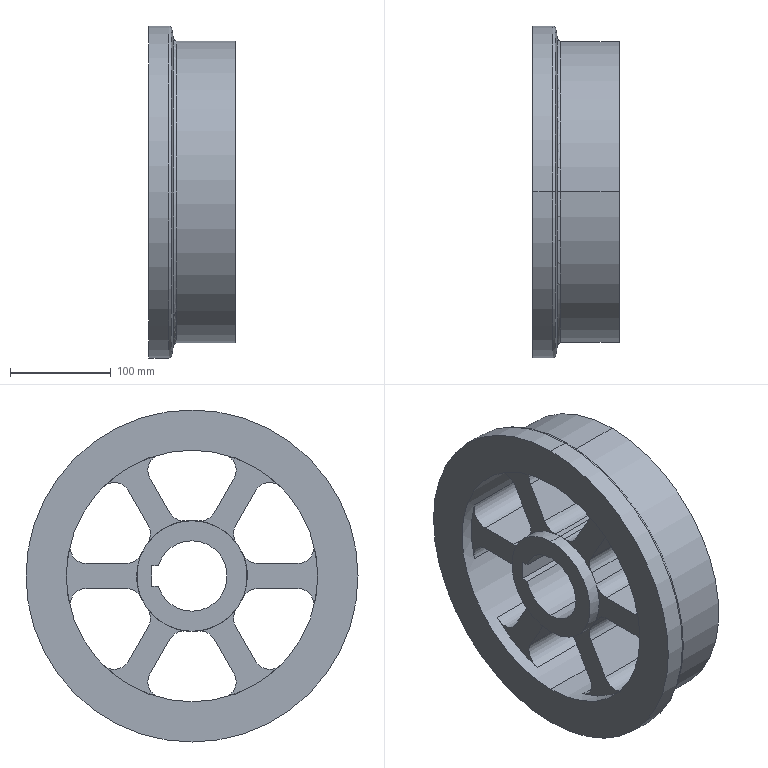Part | SolidWorks | features ICE 2, Revolution 1 | 1 solid | 78 faces | box 86 x 330 x 330 mm | volume 3397345 mm3 | cylinder 41 | plane 31 | torus 4 | cone 2 | commonest cylinder face diameters 32 x28 110 x4 70 x3 250 x2 300 x2 330 x2